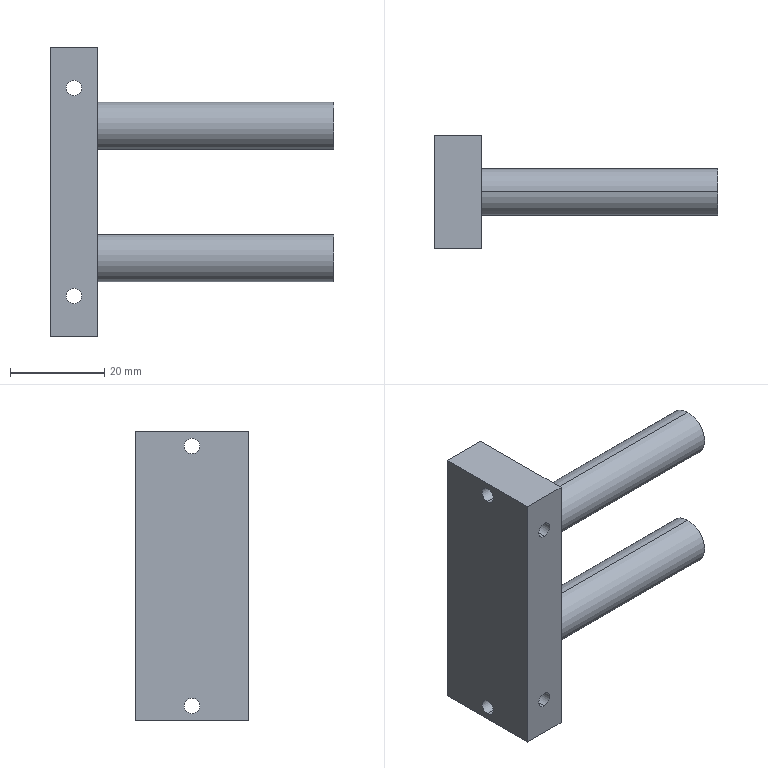Part | STEP file | PN_0013 cylinder TN-20X125 | 1 solid | 20 faces | box 60 x 24 x 61 mm | volume 21912 mm3 | cylinder 12 | plane 8 | commonest cylinder face diameters 3.3 x8 10 x4
STEP:
#1=CARTESIAN_POINT('',(0.,0.,0.));
#2=DIRECTION('',(0.,0.,1.));
#3=DIRECTION('',(1.,0.,0.));
#4=AXIS2_PLACEMENT_3D('',#1,#2,#3);
#5=CARTESIAN_POINT('',(0.,-12.,23.65));
#6=VERTEX_POINT('',#5);
#7=CARTESIAN_POINT('',(0.,12.,23.65));
#8=VERTEX_POINT('',#7);
#9=CARTESIAN_POINT('',(0.,12.,23.65));
#10=DIRECTION('',(0.,1.,0.));
#11=VECTOR('',#10,1.);
#12=LINE('',#9,#11);
#13=CARTESIAN_POINT('',(0.,12.,22.));
#14=DIRECTION('',(0.,1.,0.));
#15=DIRECTION('',(0.,0.,1.));
#16=AXIS2_PLACEMENT_3D('',#13,#14,#15);
#17=CYLINDRICAL_SURFACE('',#16,1.65);
#18=CARTESIAN_POINT('',(6.283,0.));
#19=DIRECTION('',(0.,1.));
#20=VECTOR('',#19,1.);
#21=LINE('',#18,#20);
#22=(GEOMETRIC_REPRESENTATION_CONTEXT(2)PARAMETRIC_REPRESENTATION_CONTEXT()REPRESENTATION_CONTEXT('',''));
#23=DEFINITIONAL_REPRESENTATION('',(#21),#22);
#24=PCURVE('',#17,#23);
#25=CARTESIAN_POINT('',(0.,12.,22.));
#26=DIRECTION('',(0.,1.,0.));
#27=DIRECTION('',(0.,0.,1.));
#28=AXIS2_PLACEMENT_3D('',#25,#26,#27);
#29=CYLINDRICAL_SURFACE('',#28,1.65);
#30=CARTESIAN_POINT('',(0.,0.));
#31=DIRECTION('',(0.,1.));
#32=VECTOR('',#31,1.);
#33=LINE('',#30,#32);
#34=(GEOMETRIC_REPRESENTATION_CONTEXT(2)PARAMETRIC_REPRESENTATION_CONTEXT()REPRESENTATION_CONTEXT('',''));
#35=DEFINITIONAL_REPRESENTATION('',(#33),#34);
#36=PCURVE('',#29,#35);
#37=SURFACE_CURVE('',#12,(#24,#36),.PCURVE_S1.);
#38=EDGE_CURVE('',#6,#8,#37,.T.);
#39=ORIENTED_EDGE('',*,*,#38,.T.);
#40=CARTESIAN_POINT('',(0.,12.,20.35));
#41=VERTEX_POINT('',#40);
#42=CARTESIAN_POINT('',(0.,12.,22.));
#43=DIRECTION('',(0.,1.,0.));
#44=DIRECTION('',(0.,0.,1.));
#45=AXIS2_PLACEMENT_3D('',#42,#43,#44);
#46=CIRCLE('',#45,1.65);
#47=CARTESIAN_POINT('',(0.,0.));
#48=DIRECTION('',(1.,0.));
#49=VECTOR('',#48,1.);
#50=LINE('',#47,#49);
#51=(GEOMETRIC_REPRESENTATION_CONTEXT(2)PARAMETRIC_REPRESENTATION_CONTEXT()REPRESENTATION_CONTEXT('',''));
#52=DEFINITIONAL_REPRESENTATION('',(#50),#51);
#53=PCURVE('',#17,#52);
#54=CARTESIAN_POINT('',(5.,12.,-30.5));
#55=DIRECTION('',(0.,-1.,0.));
#56=DIRECTION('',(0.,0.,-1.));
#57=AXIS2_PLACEMENT_3D('',#54,#55,#56);
#58=PLANE('',#57);
#59=CARTESIAN_POINT('',(-54.15,-5.));
#60=CARTESIAN_POINT('',(-54.15,-2.142));
#61=CARTESIAN_POINT('',(-51.675,-3.571));
#62=CARTESIAN_POINT('',(-49.2,-5.));
#63=CARTESIAN_POINT('',(-51.675,-6.429));
#64=CARTESIAN_POINT('',(-54.15,-7.858));
#65=CARTESIAN_POINT('',(-54.15,-5.));
#66=(BOUNDED_CURVE()B_SPLINE_CURVE(2,(#59,#60,#61,#62,#63,#64,#65),.UNSPECIFIED.,.T.,.F.)B_SPLINE_CURVE_WITH_KNOTS((1,2,2,2,2,1),(-2.094,0.,2.094,4.189,6.283,8.378),.UNSPECIFIED.)CURVE()GEOMETRIC_REPRESENTATION_ITEM()RATIONAL_B_SPLINE_CURVE((1.,0.5,1.,0.5,1.,0.5,1.))REPRESENTATION_ITEM(''));
#67=(GEOMETRIC_REPRESENTATION_CONTEXT(2)PARAMETRIC_REPRESENTATION_CONTEXT()REPRESENTATION_CONTEXT('',''));
#68=DEFINITIONAL_REPRESENTATION('',(#66),#67);
#69=PCURVE('',#58,#68);
#70=SURFACE_CURVE('',#46,(#53,#69),.PCURVE_S1.);
#71=EDGE_CURVE('',#41,#8,#70,.T.);
#72=ORIENTED_EDGE('',*,*,#71,.F.);
#73=CARTESIAN_POINT('',(0.,-12.,20.35));
#74=VERTEX_POINT('',#73);
#75=CARTESIAN_POINT('',(0.,12.,20.35));
#76=DIRECTION('',(0.,1.,0.));
#77=VECTOR('',#76,1.);
#78=LINE('',#75,#77);
#79=CARTESIAN_POINT('',(3.142,0.));
#80=DIRECTION('',(0.,1.));
#81=VECTOR('',#80,1.);
#82=LINE('',#79,#81);
#83=(GEOMETRIC_REPRESENTATION_CONTEXT(2)PARAMETRIC_REPRESENTATION_CONTEXT()REPRESENTATION_CONTEXT('',''));
#84=DEFINITIONAL_REPRESENTATION('',(#82),#83);
#85=PCURVE('',#17,#84);
#86=CARTESIAN_POINT('',(3.142,0.));
#87=DIRECTION('',(0.,1.));
#88=VECTOR('',#87,1.);
#89=LINE('',#86,#88);
#90=(GEOMETRIC_REPRESENTATION_CONTEXT(2)PARAMETRIC_REPRESENTATION_CONTEXT()REPRESENTATION_CONTEXT('',''));
#91=DEFINITIONAL_REPRESENTATION('',(#89),#90);
#92=PCURVE('',#29,#91);
#93=SURFACE_CURVE('',#78,(#85,#92),.PCURVE_S1.);
#94=EDGE_CURVE('',#74,#41,#93,.T.);
#95=ORIENTED_EDGE('',*,*,#94,.F.);
#96=CARTESIAN_POINT('',(0.,-12.,22.));
#97=DIRECTION('',(0.,1.,0.));
#98=DIRECTION('',(0.,0.,1.));
#99=AXIS2_PLACEMENT_3D('',#96,#97,#98);
#100=CIRCLE('',#99,1.65);
#101=CARTESIAN_POINT('',(0.,-24.));
#102=DIRECTION('',(1.,0.));
#103=VECTOR('',#102,1.);
#104=LINE('',#101,#103);
#105=(GEOMETRIC_REPRESENTATION_CONTEXT(2)PARAMETRIC_REPRESENTATION_CONTEXT()REPRESENTATION_CONTEXT('',''));
#106=DEFINITIONAL_REPRESENTATION('',(#104),#105);
#107=PCURVE('',#17,#106);
#108=CARTESIAN_POINT('',(5.,-12.,-30.5));
#109=DIRECTION('',(0.,1.,0.));
#110=DIRECTION('',(0.,0.,1.));
#111=AXIS2_PLACEMENT_3D('',#108,#109,#110);
#112=PLANE('',#111);
#113=CARTESIAN_POINT('',(52.5,-5.));
#114=DIRECTION('',(1.,0.));
#115=AXIS2_PLACEMENT_2D('',#113,#114);
#116=CIRCLE('',#115,1.65);
#117=(GEOMETRIC_REPRESENTATION_CONTEXT(2)PARAMETRIC_REPRESENTATION_CONTEXT()REPRESENTATION_CONTEXT('',''));
#118=DEFINITIONAL_REPRESENTATION('',(#116),#117);
#119=PCURVE('',#112,#118);
#120=SURFACE_CURVE('',#100,(#107,#119),.PCURVE_S1.);
#121=EDGE_CURVE('',#74,#6,#120,.T.);
#122=ORIENTED_EDGE('',*,*,#121,.T.);
#123=EDGE_LOOP('',(#39,#72,#95,#122));
#124=FACE_BOUND('',#123,.F.);
#125=ADVANCED_FACE('',(#124),#17,.F.);
#126=CARTESIAN_POINT('',(0.,-12.,-20.35));
#127=VERTEX_POINT('',#126);
#128=CARTESIAN_POINT('',(0.,12.,-20.35));
#129=VERTEX_POINT('',#128);
#130=CARTESIAN_POINT('',(0.,12.,-20.35));
#131=DIRECTION('',(0.,1.,0.));
#132=VECTOR('',#131,1.);
#133=LINE('',#130,#132);
#134=CARTESIAN_POINT('',(0.,12.,-22.));
#135=DIRECTION('',(0.,1.,0.));
#136=DIRECTION('',(0.,0.,1.));
#137=AXIS2_PLACEMENT_3D('',#134,#135,#136);
#138=CYLINDRICAL_SURFACE('',#137,1.65);
#139=CARTESIAN_POINT('',(6.283,0.));
#140=DIRECTION('',(0.,1.));
#141=VECTOR('',#140,1.);
#142=LINE('',#139,#141);
#143=(GEOMETRIC_REPRESENTATION_CONTEXT(2)PARAMETRIC_REPRESENTATION_CONTEXT()REPRESENTATION_CONTEXT('',''));
#144=DEFINITIONAL_REPRESENTATION('',(#142),#143);
#145=PCURVE('',#138,#144);
#146=CARTESIAN_POINT('',(0.,12.,-22.));
#147=DIRECTION('',(0.,1.,0.));
#148=DIRECTION('',(0.,0.,1.));
#149=AXIS2_PLACEMENT_3D('',#146,#147,#148);
#150=CYLINDRICAL_SURFACE('',#149,1.65);
#151=CARTESIAN_POINT('',(0.,0.));
#152=DIRECTION('',(0.,1.));
#153=VECTOR('',#152,1.);
#154=LINE('',#151,#153);
#155=(GEOMETRIC_REPRESENTATION_CONTEXT(2)PARAMETRIC_REPRESENTATION_CONTEXT()REPRESENTATION_CONTEXT('',''));
#156=DEFINITIONAL_REPRESENTATION('',(#154),#155);
#157=PCURVE('',#150,#156);
#158=SURFACE_CURVE('',#133,(#145,#157),.PCURVE_S1.);
#159=EDGE_CURVE('',#127,#129,#158,.T.);
#160=ORIENTED_EDGE('',*,*,#159,.T.);
#161=CARTESIAN_POINT('',(0.,12.,-23.65));
#162=VERTEX_POINT('',#161);
#163=CARTESIAN_POINT('',(0.,12.,-22.));
#164=DIRECTION('',(0.,1.,0.));
#165=DIRECTION('',(0.,0.,1.));
#166=AXIS2_PLACEMENT_3D('',#163,#164,#165);
#167=CIRCLE('',#166,1.65);
#168=CARTESIAN_POINT('',(0.,0.));
#169=DIRECTION('',(1.,0.));
#170=VECTOR('',#169,1.);
#171=LINE('',#168,#170);
#172=(GEOMETRIC_REPRESENTATION_CONTEXT(2)PARAMETRIC_REPRESENTATION_CONTEXT()REPRESENTATION_CONTEXT('',''));
#173=DEFINITIONAL_REPRESENTATION('',(#171),#172);
#174=PCURVE('',#138,#173);
#175=CARTESIAN_POINT('',(-10.15,-5.));
#176=CARTESIAN_POINT('',(-10.15,-2.142));
#177=CARTESIAN_POINT('',(-7.675,-3.571));
#178=CARTESIAN_POINT('',(-5.2,-5.));
#179=CARTESIAN_POINT('',(-7.675,-6.429));
#180=CARTESIAN_POINT('',(-10.15,-7.858));
#181=CARTESIAN_POINT('',(-10.15,-5.));
#182=(BOUNDED_CURVE()B_SPLINE_CURVE(2,(#175,#176,#177,#178,#179,#180,#181),.UNSPECIFIED.,.T.,.F.)B_SPLINE_CURVE_WITH_KNOTS((1,2,2,2,2,1),(-2.094,0.,2.094,4.189,6.283,8.378),.UNSPECIFIED.)CURVE()GEOMETRIC_REPRESENTATION_ITEM()RATIONAL_B_SPLINE_CURVE((1.,0.5,1.,0.5,1.,0.5,1.))REPRESENTATION_ITEM(''));
#183=(GEOMETRIC_REPRESENTATION_CONTEXT(2)PARAMETRIC_REPRESENTATION_CONTEXT()REPRESENTATION_CONTEXT('',''));
#184=DEFINITIONAL_REPRESENTATION('',(#182),#183);
#185=PCURVE('',#58,#184);
#186=SURFACE_CURVE('',#167,(#174,#185),.PCURVE_S1.);
#187=EDGE_CURVE('',#162,#129,#186,.T.);
#188=ORIENTED_EDGE('',*,*,#187,.F.);
#189=CARTESIAN_POINT('',(0.,-12.,-23.65));
#190=VERTEX_POINT('',#189);
#191=CARTESIAN_POINT('',(0.,12.,-23.65));
#192=DIRECTION('',(0.,1.,0.));
#193=VECTOR('',#192,1.);
#194=LINE('',#191,#193);
#195=CARTESIAN_POINT('',(3.142,0.));
#196=DIRECTION('',(0.,1.));
#197=VECTOR('',#196,1.);
#198=LINE('',#195,#197);
#199=(GEOMETRIC_REPRESENTATION_CONTEXT(2)PARAMETRIC_REPRESENTATION_CONTEXT()REPRESENTATION_CONTEXT('',''));
#200=DEFINITIONAL_REPRESENTATION('',(#198),#199);
#201=PCURVE('',#138,#200);
#202=CARTESIAN_POINT('',(3.142,0.));
#203=DIRECTION('',(0.,1.));
#204=VECTOR('',#203,1.);
#205=LINE('',#202,#204);
#206=(GEOMETRIC_REPRESENTATION_CONTEXT(2)PARAMETRIC_REPRESENTATION_CONTEXT()REPRESENTATION_CONTEXT('',''));
#207=DEFINITIONAL_REPRESENTATION('',(#205),#206);
#208=PCURVE('',#150,#207);
#209=SURFACE_CURVE('',#194,(#201,#208),.PCURVE_S1.);
#210=EDGE_CURVE('',#190,#162,#209,.T.);
#211=ORIENTED_EDGE('',*,*,#210,.F.);
#212=CARTESIAN_POINT('',(0.,-12.,-22.));
#213=DIRECTION('',(0.,1.,0.));
#214=DIRECTION('',(0.,0.,1.));
#215=AXIS2_PLACEMENT_3D('',#212,#213,#214);
#216=CIRCLE('',#215,1.65);
#217=CARTESIAN_POINT('',(0.,-24.));
#218=DIRECTION('',(1.,0.));
#219=VECTOR('',#218,1.);
#220=LINE('',#217,#219);
#221=(GEOMETRIC_REPRESENTATION_CONTEXT(2)PARAMETRIC_REPRESENTATION_CONTEXT()REPRESENTATION_CONTEXT('',''));
#222=DEFINITIONAL_REPRESENTATION('',(#220),#221);
#223=PCURVE('',#138,#222);
#224=CARTESIAN_POINT('',(8.5,-5.));
#225=DIRECTION('',(1.,0.));
#226=AXIS2_PLACEMENT_2D('',#224,#225);
#227=CIRCLE('',#226,1.65);
#228=(GEOMETRIC_REPRESENTATION_CONTEXT(2)PARAMETRIC_REPRESENTATION_CONTEXT()REPRESENTATION_CONTEXT('',''));
#229=DEFINITIONAL_REPRESENTATION('',(#227),#228);
#230=PCURVE('',#112,#229);
#231=SURFACE_CURVE('',#216,(#223,#230),.PCURVE_S1.);
#232=EDGE_CURVE('',#190,#127,#231,.T.);
#233=ORIENTED_EDGE('',*,*,#232,.T.);
#234=EDGE_LOOP('',(#160,#188,#211,#233));
#235=FACE_BOUND('',#234,.F.);
#236=ADVANCED_FACE('',(#235),#138,.F.);
#237=CARTESIAN_POINT('',(5.,0.,-25.85));
#238=VERTEX_POINT('',#237);
#239=CARTESIAN_POINT('',(-5.,0.,-25.85));
#240=VERTEX_POINT('',#239);
#241=CARTESIAN_POINT('',(-5.,0.,-25.85));
#242=DIRECTION('',(-1.,0.,0.));
#243=VECTOR('',#242,1.);
#244=LINE('',#241,#243);
#245=CARTESIAN_POINT('',(-5.,0.,-27.5));
#246=DIRECTION('',(-1.,0.,0.));
#247=DIRECTION('',(0.,0.,1.));
#248=AXIS2_PLACEMENT_3D('',#245,#246,#247);
#249=CYLINDRICAL_SURFACE('',#248,1.65);
#250=CARTESIAN_POINT('',(6.283,0.));
#251=DIRECTION('',(0.,1.));
#252=VECTOR('',#251,1.);
#253=LINE('',#250,#252);
#254=(GEOMETRIC_REPRESENTATION_CONTEXT(2)PARAMETRIC_REPRESENTATION_CONTEXT()REPRESENTATION_CONTEXT('',''));
#255=DEFINITIONAL_REPRESENTATION('',(#253),#254);
#256=PCURVE('',#249,#255);
#257=CARTESIAN_POINT('',(-5.,0.,-27.5));
#258=DIRECTION('',(-1.,0.,0.));
#259=DIRECTION('',(0.,0.,1.));
#260=AXIS2_PLACEMENT_3D('',#257,#258,#259);
#261=CYLINDRICAL_SURFACE('',#260,1.65);
#262=CARTESIAN_POINT('',(0.,0.));
#263=DIRECTION('',(0.,1.));
#264=VECTOR('',#263,1.);
#265=LINE('',#262,#264);
#266=(GEOMETRIC_REPRESENTATION_CONTEXT(2)PARAMETRIC_REPRESENTATION_CONTEXT()REPRESENTATION_CONTEXT('',''));
#267=DEFINITIONAL_REPRESENTATION('',(#265),#266);
#268=PCURVE('',#261,#267);
#269=SURFACE_CURVE('',#244,(#256,#268),.PCURVE_S1.);
#270=EDGE_CURVE('',#238,#240,#269,.T.);
#271=ORIENTED_EDGE('',*,*,#270,.T.);
#272=CARTESIAN_POINT('',(-5.,0.,-29.15));
#273=VERTEX_POINT('',#272);
#274=CARTESIAN_POINT('',(-5.,0.,-27.5));
#275=DIRECTION('',(-1.,0.,0.));
#276=DIRECTION('',(0.,0.,1.));
#277=AXIS2_PLACEMENT_3D('',#274,#275,#276);
#278=CIRCLE('',#277,1.65);
#279=CARTESIAN_POINT('',(0.,0.));
#280=DIRECTION('',(1.,0.));
#281=VECTOR('',#280,1.);
#282=LINE('',#279,#281);
#283=(GEOMETRIC_REPRESENTATION_CONTEXT(2)PARAMETRIC_REPRESENTATION_CONTEXT()REPRESENTATION_CONTEXT('',''));
#284=DEFINITIONAL_REPRESENTATION('',(#282),#283);
#285=PCURVE('',#249,#284);
#286=CARTESIAN_POINT('',(-5.,0.,0.));
#287=DIRECTION('',(1.,0.,0.));
#288=DIRECTION('',(0.,0.,-1.));
#289=AXIS2_PLACEMENT_3D('',#286,#287,#288);
#290=PLANE('',#289);
#291=CARTESIAN_POINT('',(25.85,0.));
#292=CARTESIAN_POINT('',(25.85,2.858));
#293=CARTESIAN_POINT('',(28.325,1.429));
#294=CARTESIAN_POINT('',(30.8,0.));
#295=CARTESIAN_POINT('',(28.325,-1.429));
#296=CARTESIAN_POINT('',(25.85,-2.858));
#297=CARTESIAN_POINT('',(25.85,0.));
#298=(BOUNDED_CURVE()B_SPLINE_CURVE(2,(#291,#292,#293,#294,#295,#296,#297),.UNSPECIFIED.,.T.,.F.)B_SPLINE_CURVE_WITH_KNOTS((1,2,2,2,2,1),(-2.094,0.,2.094,4.189,6.283,8.378),.UNSPECIFIED.)CURVE()GEOMETRIC_REPRESENTATION_ITEM()RATIONAL_B_SPLINE_CURVE((1.,0.5,1.,0.5,1.,0.5,1.))REPRESENTATION_ITEM(''));
#299=(GEOMETRIC_REPRESENTATION_CONTEXT(2)PARAMETRIC_REPRESENTATION_CONTEXT()REPRESENTATION_CONTEXT('',''));
#300=DEFINITIONAL_REPRESENTATION('',(#298),#299);
#301=PCURVE('',#290,#300);
#302=SURFACE_CURVE('',#278,(#285,#301),.PCURVE_S1.);
#303=EDGE_CURVE('',#273,#240,#302,.T.);
#304=ORIENTED_EDGE('',*,*,#303,.F.);
#305=CARTESIAN_POINT('',(5.,0.,-29.15));
#306=VERTEX_POINT('',#305);
#307=CARTESIAN_POINT('',(-5.,0.,-29.15));
#308=DIRECTION('',(-1.,0.,0.));
#309=VECTOR('',#308,1.);
#310=LINE('',#307,#309);
#311=CARTESIAN_POINT('',(3.142,0.));
#312=DIRECTION('',(0.,1.));
#313=VECTOR('',#312,1.);
#314=LINE('',#311,#313);
#315=(GEOMETRIC_REPRESENTATION_CONTEXT(2)PARAMETRIC_REPRESENTATION_CONTEXT()REPRESENTATION_CONTEXT('',''));
#316=DEFINITIONAL_REPRESENTATION('',(#314),#315);
#317=PCURVE('',#249,#316);
#318=CARTESIAN_POINT('',(3.142,0.));
#319=DIRECTION('',(0.,1.));
#320=VECTOR('',#319,1.);
#321=LINE('',#318,#320);
#322=(GEOMETRIC_REPRESENTATION_CONTEXT(2)PARAMETRIC_REPRESENTATION_CONTEXT()REPRESENTATION_CONTEXT('',''));
#323=DEFINITIONAL_REPRESENTATION('',(#321),#322);
#324=PCURVE('',#261,#323);
#325=SURFACE_CURVE('',#310,(#317,#324),.PCURVE_S1.);
#326=EDGE_CURVE('',#306,#273,#325,.T.);
#327=ORIENTED_EDGE('',*,*,#326,.F.);
#328=CARTESIAN_POINT('',(5.,0.,-27.5));
#329=DIRECTION('',(1.,0.,0.));
#330=DIRECTION('',(0.,0.,-1.));
#331=AXIS2_PLACEMENT_3D('',#328,#329,#330);
#332=CIRCLE('',#331,1.65);
#333=CARTESIAN_POINT('',(9.425,-10.));
#334=DIRECTION('',(-1.,0.));
#335=VECTOR('',#334,1.);
#336=LINE('',#333,#335);
#337=(GEOMETRIC_REPRESENTATION_CONTEXT(2)PARAMETRIC_REPRESENTATION_CONTEXT()REPRESENTATION_CONTEXT('',''));
#338=DEFINITIONAL_REPRESENTATION('',(#336),#337);
#339=PCURVE('',#249,#338);
#340=CARTESIAN_POINT('',(5.,0.,0.));
#341=DIRECTION('',(1.,0.,0.));
#342=DIRECTION('',(0.,0.,-1.));
#343=AXIS2_PLACEMENT_3D('',#340,#341,#342);
#344=PLANE('',#343);
#345=CARTESIAN_POINT('',(27.5,0.));
#346=DIRECTION('',(1.,0.));
#347=AXIS2_PLACEMENT_2D('',#345,#346);
#348=CIRCLE('',#347,1.65);
#349=(GEOMETRIC_REPRESENTATION_CONTEXT(2)PARAMETRIC_REPRESENTATION_CONTEXT()REPRESENTATION_CONTEXT('',''));
#350=DEFINITIONAL_REPRESENTATION('',(#348),#349);
#351=PCURVE('',#344,#350);
#352=SURFACE_CURVE('',#332,(#339,#351),.PCURVE_S1.);
#353=EDGE_CURVE('',#238,#306,#352,.T.);
#354=ORIENTED_EDGE('',*,*,#353,.F.);
#355=EDGE_LOOP('',(#271,#304,#327,#354));
#356=FACE_BOUND('',#355,.F.);
#357=ADVANCED_FACE('',(#356),#249,.F.);
#358=CARTESIAN_POINT('',(5.,0.,29.15));
#359=VERTEX_POINT('',#358);
#360=CARTESIAN_POINT('',(-5.,0.,29.15));
#361=VERTEX_POINT('',#360);
#362=CARTESIAN_POINT('',(-5.,0.,29.15));
#363=DIRECTION('',(-1.,0.,0.));
#364=VECTOR('',#363,1.);
#365=LINE('',#362,#364);
#366=CARTESIAN_POINT('',(-5.,0.,27.5));
#367=DIRECTION('',(-1.,0.,0.));
#368=DIRECTION('',(0.,0.,1.));
#369=AXIS2_PLACEMENT_3D('',#366,#367,#368);
#370=CYLINDRICAL_SURFACE('',#369,1.65);
#371=CARTESIAN_POINT('',(6.283,0.));
#372=DIRECTION('',(0.,1.));
#373=VECTOR('',#372,1.);
#374=LINE('',#371,#373);
#375=(GEOMETRIC_REPRESENTATION_CONTEXT(2)PARAMETRIC_REPRESENTATION_CONTEXT()REPRESENTATION_CONTEXT('',''));
#376=DEFINITIONAL_REPRESENTATION('',(#374),#375);
#377=PCURVE('',#370,#376);
#378=CARTESIAN_POINT('',(-5.,0.,27.5));
#379=DIRECTION('',(-1.,0.,0.));
#380=DIRECTION('',(0.,0.,1.));
#381=AXIS2_PLACEMENT_3D('',#378,#379,#380);
#382=CYLINDRICAL_SURFACE('',#381,1.65);
#383=CARTESIAN_POINT('',(0.,0.));
#384=DIRECTION('',(0.,1.));
#385=VECTOR('',#384,1.);
#386=LINE('',#383,#385);
#387=(GEOMETRIC_REPRESENTATION_CONTEXT(2)PARAMETRIC_REPRESENTATION_CONTEXT()REPRESENTATION_CONTEXT('',''));
#388=DEFINITIONAL_REPRESENTATION('',(#386),#387);
#389=PCURVE('',#382,#388);
#390=SURFACE_CURVE('',#365,(#377,#389),.PCURVE_S1.);
#391=EDGE_CURVE('',#359,#361,#390,.T.);
#392=ORIENTED_EDGE('',*,*,#391,.T.);
#393=CARTESIAN_POINT('',(-5.,0.,25.85));
#394=VERTEX_POINT('',#393);
#395=CARTESIAN_POINT('',(-5.,0.,27.5));
#396=DIRECTION('',(-1.,0.,0.));
#397=DIRECTION('',(0.,0.,1.));
#398=AXIS2_PLACEMENT_3D('',#395,#396,#397);
#399=CIRCLE('',#398,1.65);
#400=CARTESIAN_POINT('',(0.,0.));
#401=DIRECTION('',(1.,0.));
#402=VECTOR('',#401,1.);
#403=LINE('',#400,#402);
#404=(GEOMETRIC_REPRESENTATION_CONTEXT(2)PARAMETRIC_REPRESENTATION_CONTEXT()REPRESENTATION_CONTEXT('',''));
#405=DEFINITIONAL_REPRESENTATION('',(#403),#404);
#406=PCURVE('',#370,#405);
#407=CARTESIAN_POINT('',(-29.15,0.));
#408=CARTESIAN_POINT('',(-29.15,2.858));
#409=CARTESIAN_POINT('',(-26.675,1.429));
#410=CARTESIAN_POINT('',(-24.2,0.));
#411=CARTESIAN_POINT('',(-26.675,-1.429));
#412=CARTESIAN_POINT('',(-29.15,-2.858));
#413=CARTESIAN_POINT('',(-29.15,0.));
#414=(BOUNDED_CURVE()B_SPLINE_CURVE(2,(#407,#408,#409,#410,#411,#412,#413),.UNSPECIFIED.,.T.,.F.)B_SPLINE_CURVE_WITH_KNOTS((1,2,2,2,2,1),(-2.094,0.,2.094,4.189,6.283,8.378),.UNSPECIFIED.)CURVE()GEOMETRIC_REPRESENTATION_ITEM()RATIONAL_B_SPLINE_CURVE((1.,0.5,1.,0.5,1.,0.5,1.))REPRESENTATION_ITEM(''));
#415=(GEOMETRIC_REPRESENTATION_CONTEXT(2)PARAMETRIC_REPRESENTATION_CONTEXT()REPRESENTATION_CONTEXT('',''));
#416=DEFINITIONAL_REPRESENTATION('',(#414),#415);
#417=PCURVE('',#290,#416);
#418=SURFACE_CURVE('',#399,(#406,#417),.PCURVE_S1.);
#419=EDGE_CURVE('',#394,#361,#418,.T.);
#420=ORIENTED_EDGE('',*,*,#419,.F.);
#421=CARTESIAN_POINT('',(5.,0.,25.85));
#422=VERTEX_POINT('',#421);
#423=CARTESIAN_POINT('',(-5.,0.,25.85));
#424=DIRECTION('',(-1.,0.,0.));
#425=VECTOR('',#424,1.);
#426=LINE('',#423,#425);
#427=CARTESIAN_POINT('',(3.142,0.));
#428=DIRECTION('',(0.,1.));
#429=VECTOR('',#428,1.);
#430=LINE('',#427,#429);
#431=(GEOMETRIC_REPRESENTATION_CONTEXT(2)PARAMETRIC_REPRESENTATION_CONTEXT()REPRESENTATION_CONTEXT('',''));
#432=DEFINITIONAL_REPRESENTATION('',(#430),#431);
#433=PCURVE('',#370,#432);
#434=CARTESIAN_POINT('',(3.142,0.));
#435=DIRECTION('',(0.,1.));
#436=VECTOR('',#435,1.);
#437=LINE('',#434,#436);
#438=(GEOMETRIC_REPRESENTATION_CONTEXT(2)PARAMETRIC_REPRESENTATION_CONTEXT()REPRESENTATION_CONTEXT('',''));
#439=DEFINITIONAL_REPRESENTATION('',(#437),#438);
#440=PCURVE('',#382,#439);
#441=SURFACE_CURVE('',#426,(#433,#440),.PCURVE_S1.);
#442=EDGE_CURVE('',#422,#394,#441,.T.);
#443=ORIENTED_EDGE('',*,*,#442,.F.);
#444=CARTESIAN_POINT('',(5.,0.,27.5));
#445=DIRECTION('',(1.,0.,0.));
#446=DIRECTION('',(0.,0.,-1.));
#447=AXIS2_PLACEMENT_3D('',#444,#445,#446);
#448=CIRCLE('',#447,1.65);
#449=CARTESIAN_POINT('',(9.425,-10.));
#450=DIRECTION('',(-1.,0.));
#451=VECTOR('',#450,1.);
#452=LINE('',#449,#451);
#453=(GEOMETRIC_REPRESENTATION_CONTEXT(2)PARAMETRIC_REPRESENTATION_CONTEXT()REPRESENTATION_CONTEXT('',''));
#454=DEFINITIONAL_REPRESENTATION('',(#452),#453);
#455=PCURVE('',#370,#454);
#456=CARTESIAN_POINT('',(-27.5,0.));
#457=DIRECTION('',(1.,0.));
#458=AXIS2_PLACEMENT_2D('',#456,#457);
#459=CIRCLE('',#458,1.65);
#460=(GEOMETRIC_REPRESENTATION_CONTEXT(2)PARAMETRIC_REPRESENTATION_CONTEXT()REPRESENTATION_CONTEXT('',''));
#461=DEFINITIONAL_REPRESENTATION('',(#459),#460);
#462=PCURVE('',#344,#461);
#463=SURFACE_CURVE('',#448,(#455,#462),.PCURVE_S1.);
#464=EDGE_CURVE('',#359,#422,#463,.T.);
#465=ORIENTED_EDGE('',*,*,#464,.F.);
#466=EDGE_LOOP('',(#392,#420,#443,#465));
#467=FACE_BOUND('',#466,.F.);
#468=ADVANCED_FACE('',(#467),#370,.F.);
#469=CARTESIAN_POINT('',(55.,0.,-19.));
#470=VERTEX_POINT('',#469);
#471=CARTESIAN_POINT('',(55.,0.,-9.));
#472=VERTEX_POINT('',#471);
#473=CARTESIAN_POINT('',(55.,0.,-14.));
#474=DIRECTION('',(1.,0.,0.));
#475=DIRECTION('',(0.,0.,-1.));
#476=AXIS2_PLACEMENT_3D('',#473,#474,#475);
#477=CIRCLE('',#476,5.);
#478=CARTESIAN_POINT('',(55.,0.,-14.));
#479=DIRECTION('',(-1.,0.,0.));
#480=DIRECTION('',(0.,0.,1.));
#481=AXIS2_PLACEMENT_3D('',#478,#479,#480);
#482=CYLINDRICAL_SURFACE('',#481,5.);
#483=CARTESIAN_POINT('',(3.142,0.));
#484=DIRECTION('',(-1.,0.));
#485=VECTOR('',#484,1.);
#486=LINE('',#483,#485);
#487=(GEOMETRIC_REPRESENTATION_CONTEXT(2)PARAMETRIC_REPRESENTATION_CONTEXT()REPRESENTATION_CONTEXT('',''));
#488=DEFINITIONAL_REPRESENTATION('',(#486),#487);
#489=PCURVE('',#482,#488);
#490=CARTESIAN_POINT('',(55.,0.,-14.));
#491=DIRECTION('',(1.,0.,0.));
#492=DIRECTION('',(0.,0.,-1.));
#493=AXIS2_PLACEMENT_3D('',#490,#491,#492);
#494=PLANE('',#493);
#495=CARTESIAN_POINT('',(0.,0.));
#496=DIRECTION('',(1.,0.));
#497=AXIS2_PLACEMENT_2D('',#495,#496);
#498=CIRCLE('',#497,5.);
#499=(GEOMETRIC_REPRESENTATION_CONTEXT(2)PARAMETRIC_REPRESENTATION_CONTEXT()REPRESENTATION_CONTEXT('',''));
#500=DEFINITIONAL_REPRESENTATION('',(#498),#499);
#501=PCURVE('',#494,#500);
#502=SURFACE_CURVE('',#477,(#489,#501),.PCURVE_S1.);
#503=EDGE_CURVE('',#470,#472,#502,.T.);
#504=ORIENTED_EDGE('',*,*,#503,.F.);
#505=CARTESIAN_POINT('',(5.,0.,-19.));
#506=VERTEX_POINT('',#505);
#507=CARTESIAN_POINT('',(55.,0.,-19.));
#508=DIRECTION('',(-1.,0.,0.));
#509=VECTOR('',#508,1.);
#510=LINE('',#507,#509);
#511=CARTESIAN_POINT('',(3.142,0.));
#512=DIRECTION('',(0.,1.));
#513=VECTOR('',#512,1.);
#514=LINE('',#511,#513);
#515=(GEOMETRIC_REPRESENTATION_CONTEXT(2)PARAMETRIC_REPRESENTATION_CONTEXT()REPRESENTATION_CONTEXT('',''));
#516=DEFINITIONAL_REPRESENTATION('',(#514),#515);
#517=PCURVE('',#482,#516);
#518=CARTESIAN_POINT('',(55.,0.,-14.));
#519=DIRECTION('',(-1.,0.,0.));
#520=DIRECTION('',(0.,0.,1.));
#521=AXIS2_PLACEMENT_3D('',#518,#519,#520);
#522=CYLINDRICAL_SURFACE('',#521,5.);
#523=CARTESIAN_POINT('',(3.142,0.));
#524=DIRECTION('',(0.,1.));
#525=VECTOR('',#524,1.);
#526=LINE('',#523,#525);
#527=(GEOMETRIC_REPRESENTATION_CONTEXT(2)PARAMETRIC_REPRESENTATION_CONTEXT()REPRESENTATION_CONTEXT('',''));
#528=DEFINITIONAL_REPRESENTATION('',(#526),#527);
#529=PCURVE('',#522,#528);
#530=SURFACE_CURVE('',#510,(#517,#529),.PCURVE_S1.);
#531=EDGE_CURVE('',#470,#506,#530,.T.);
#532=ORIENTED_EDGE('',*,*,#531,.T.);
#533=CARTESIAN_POINT('',(5.,0.,-9.));
#534=VERTEX_POINT('',#533);
#535=CARTESIAN_POINT('',(5.,0.,-14.));
#536=DIRECTION('',(1.,0.,0.));
#537=DIRECTION('',(0.,0.,-1.));
#538=AXIS2_PLACEMENT_3D('',#535,#536,#537);
#539=CIRCLE('',#538,5.);
#540=CARTESIAN_POINT('',(3.142,50.));
#541=DIRECTION('',(-1.,0.));
#542=VECTOR('',#541,1.);
#543=LINE('',#540,#542);
#544=(GEOMETRIC_REPRESENTATION_CONTEXT(2)PARAMETRIC_REPRESENTATION_CONTEXT()REPRESENTATION_CONTEXT('',''));
#545=DEFINITIONAL_REPRESENTATION('',(#543),#544);
#546=PCURVE('',#482,#545);
#547=CARTESIAN_POINT('',(14.,0.));
#548=DIRECTION('',(1.,0.));
#549=AXIS2_PLACEMENT_2D('',#547,#548);
#550=CIRCLE('',#549,5.);
#551=(GEOMETRIC_REPRESENTATION_CONTEXT(2)PARAMETRIC_REPRESENTATION_CONTEXT()REPRESENTATION_CONTEXT('',''));
#552=DEFINITIONAL_REPRESENTATION('',(#550),#551);
#553=PCURVE('',#344,#552);
#554=SURFACE_CURVE('',#539,(#546,#553),.PCURVE_S1.);
#555=EDGE_CURVE('',#506,#534,#554,.T.);
#556=ORIENTED_EDGE('',*,*,#555,.T.);
#557=CARTESIAN_POINT('',(55.,0.,-9.));
#558=DIRECTION('',(-1.,0.,0.));
#559=VECTOR('',#558,1.);
#560=LINE('',#557,#559);
#561=CARTESIAN_POINT('',(0.,0.));
#562=DIRECTION('',(0.,1.));
#563=VECTOR('',#562,1.);
#564=LINE('',#561,#563);
#565=(GEOMETRIC_REPRESENTATION_CONTEXT(2)PARAMETRIC_REPRESENTATION_CONTEXT()REPRESENTATION_CONTEXT('',''));
#566=DEFINITIONAL_REPRESENTATION('',(#564),#565);
#567=PCURVE('',#482,#566);
#568=CARTESIAN_POINT('',(6.283,0.));
#569=DIRECTION('',(0.,1.));
#570=VECTOR('',#569,1.);
#571=LINE('',#568,#570);
#572=(GEOMETRIC_REPRESENTATION_CONTEXT(2)PARAMETRIC_REPRESENTATION_CONTEXT()REPRESENTATION_CONTEXT('',''));
#573=DEFINITIONAL_REPRESENTATION('',(#571),#572);
#574=PCURVE('',#522,#573);
#575=SURFACE_CURVE('',#560,(#567,#574),.PCURVE_S1.);
#576=EDGE_CURVE('',#472,#534,#575,.T.);
#577=ORIENTED_EDGE('',*,*,#576,.F.);
#578=EDGE_LOOP('',(#504,#532,#556,#577));
#579=FACE_BOUND('',#578,.T.);
#580=ADVANCED_FACE('',(#579),#482,.T.);
#581=CARTESIAN_POINT('',(55.,0.,9.));
#582=VERTEX_POINT('',#581);
#583=CARTESIAN_POINT('',(55.,0.,19.));
#584=VERTEX_POINT('',#583);
#585=CARTESIAN_POINT('',(55.,0.,14.));
#586=DIRECTION('',(1.,0.,0.));
#587=DIRECTION('',(0.,0.,-1.));
#588=AXIS2_PLACEMENT_3D('',#585,#586,#587);
#589=CIRCLE('',#588,5.);
#590=CARTESIAN_POINT('',(55.,0.,14.));
#591=DIRECTION('',(-1.,0.,0.));
#592=DIRECTION('',(0.,0.,1.));
#593=AXIS2_PLACEMENT_3D('',#590,#591,#592);
#594=CYLINDRICAL_SURFACE('',#593,5.);
#595=CARTESIAN_POINT('',(3.142,0.));
#596=DIRECTION('',(-1.,0.));
#597=VECTOR('',#596,1.);
#598=LINE('',#595,#597);
#599=(GEOMETRIC_REPRESENTATION_CONTEXT(2)PARAMETRIC_REPRESENTATION_CONTEXT()REPRESENTATION_CONTEXT('',''));
#600=DEFINITIONAL_REPRESENTATION('',(#598),#599);
#601=PCURVE('',#594,#600);
#602=CARTESIAN_POINT('',(55.,0.,14.));
#603=DIRECTION('',(1.,0.,0.));
#604=DIRECTION('',(0.,0.,-1.));
#605=AXIS2_PLACEMENT_3D('',#602,#603,#604);
#606=PLANE('',#605);
#607=CARTESIAN_POINT('',(0.,0.));
#608=DIRECTION('',(1.,0.));
#609=AXIS2_PLACEMENT_2D('',#607,#608);
#610=CIRCLE('',#609,5.);
#611=(GEOMETRIC_REPRESENTATION_CONTEXT(2)PARAMETRIC_REPRESENTATION_CONTEXT()REPRESENTATION_CONTEXT('',''));
#612=DEFINITIONAL_REPRESENTATION('',(#610),#611);
#613=PCURVE('',#606,#612);
#614=SURFACE_CURVE('',#589,(#601,#613),.PCURVE_S1.);
#615=EDGE_CURVE('',#582,#584,#614,.T.);
#616=ORIENTED_EDGE('',*,*,#615,.F.);
#617=CARTESIAN_POINT('',(5.,0.,9.));
#618=VERTEX_POINT('',#617);
#619=CARTESIAN_POINT('',(55.,0.,9.));
#620=DIRECTION('',(-1.,0.,0.));
#621=VECTOR('',#620,1.);
#622=LINE('',#619,#621);
#623=CARTESIAN_POINT('',(3.142,0.));
#624=DIRECTION('',(0.,1.));
#625=VECTOR('',#624,1.);
#626=LINE('',#623,#625);
#627=(GEOMETRIC_REPRESENTATION_CONTEXT(2)PARAMETRIC_REPRESENTATION_CONTEXT()REPRESENTATION_CONTEXT('',''));
#628=DEFINITIONAL_REPRESENTATION('',(#626),#627);
#629=PCURVE('',#594,#628);
#630=CARTESIAN_POINT('',(55.,0.,14.));
#631=DIRECTION('',(-1.,0.,0.));
#632=DIRECTION('',(0.,0.,1.));
#633=AXIS2_PLACEMENT_3D('',#630,#631,#632);
#634=CYLINDRICAL_SURFACE('',#633,5.);
#635=CARTESIAN_POINT('',(3.142,0.));
#636=DIRECTION('',(0.,1.));
#637=VECTOR('',#636,1.);
#638=LINE('',#635,#637);
#639=(GEOMETRIC_REPRESENTATION_CONTEXT(2)PARAMETRIC_REPRESENTATION_CONTEXT()REPRESENTATION_CONTEXT('',''));
#640=DEFINITIONAL_REPRESENTATION('',(#638),#639);
#641=PCURVE('',#634,#640);
#642=SURFACE_CURVE('',#622,(#629,#641),.PCURVE_S1.);
#643=EDGE_CURVE('',#582,#618,#642,.T.);
#644=ORIENTED_EDGE('',*,*,#643,.T.);
#645=CARTESIAN_POINT('',(5.,0.,19.));
#646=VERTEX_POINT('',#645);
#647=CARTESIAN_POINT('',(5.,0.,14.));
#648=DIRECTION('',(1.,0.,0.));
#649=DIRECTION('',(0.,0.,-1.));
#650=AXIS2_PLACEMENT_3D('',#647,#648,#649);
#651=CIRCLE('',#650,5.);
#652=CARTESIAN_POINT('',(3.142,50.));
#653=DIRECTION('',(-1.,0.));
#654=VECTOR('',#653,1.);
#655=LINE('',#652,#654);
#656=(GEOMETRIC_REPRESENTATION_CONTEXT(2)PARAMETRIC_REPRESENTATION_CONTEXT()REPRESENTATION_CONTEXT('',''));
#657=DEFINITIONAL_REPRESENTATION('',(#655),#656);
#658=PCURVE('',#594,#657);
#659=CARTESIAN_POINT('',(-14.,0.));
#660=DIRECTION('',(1.,0.));
#661=AXIS2_PLACEMENT_2D('',#659,#660);
#662=CIRCLE('',#661,5.);
#663=(GEOMETRIC_REPRESENTATION_CONTEXT(2)PARAMETRIC_REPRESENTATION_CONTEXT()REPRESENTATION_CONTEXT('',''));
#664=DEFINITIONAL_REPRESENTATION('',(#662),#663);
#665=PCURVE('',#344,#664);
#666=SURFACE_CURVE('',#651,(#658,#665),.PCURVE_S1.);
#667=EDGE_CURVE('',#618,#646,#666,.T.);
#668=ORIENTED_EDGE('',*,*,#667,.T.);
#669=CARTESIAN_POINT('',(55.,0.,19.));
#670=DIRECTION('',(-1.,0.,0.));
#671=VECTOR('',#670,1.);
#672=LINE('',#669,#671);
#673=CARTESIAN_POINT('',(0.,0.));
#674=DIRECTION('',(0.,1.));
#675=VECTOR('',#674,1.);
#676=LINE('',#673,#675);
#677=(GEOMETRIC_REPRESENTATION_CONTEXT(2)PARAMETRIC_REPRESENTATION_CONTEXT()REPRESENTATION_CONTEXT('',''));
#678=DEFINITIONAL_REPRESENTATION('',(#676),#677);
#679=PCURVE('',#594,#678);
#680=CARTESIAN_POINT('',(6.283,0.));
#681=DIRECTION('',(0.,1.));
#682=VECTOR('',#681,1.);
#683=LINE('',#680,#682);
#684=(GEOMETRIC_REPRESENTATION_CONTEXT(2)PARAMETRIC_REPRESENTATION_CONTEXT()REPRESENTATION_CONTEXT('',''));
#685=DEFINITIONAL_REPRESENTATION('',(#683),#684);
#686=PCURVE('',#634,#685);
#687=SURFACE_CURVE('',#672,(#679,#686),.PCURVE_S1.);
#688=EDGE_CURVE('',#584,#646,#687,.T.);
#689=ORIENTED_EDGE('',*,*,#688,.F.);
#690=EDGE_LOOP('',(#616,#644,#668,#689));
#691=FACE_BOUND('',#690,.T.);
#692=ADVANCED_FACE('',(#691),#594,.T.);
#693=ORIENTED_EDGE('',*,*,#353,.F.);
#694=CARTESIAN_POINT('',(5.,0.,-27.5));
#695=DIRECTION('',(1.,0.,0.));
#696=DIRECTION('',(0.,0.,-1.));
#697=AXIS2_PLACEMENT_3D('',#694,#695,#696);
#698=CIRCLE('',#697,1.65);
#699=CARTESIAN_POINT('',(27.5,0.));
#700=DIRECTION('',(1.,0.));
#701=AXIS2_PLACEMENT_2D('',#699,#700);
#702=CIRCLE('',#701,1.65);
#703=(GEOMETRIC_REPRESENTATION_CONTEXT(2)PARAMETRIC_REPRESENTATION_CONTEXT()REPRESENTATION_CONTEXT('',''));
#704=DEFINITIONAL_REPRESENTATION('',(#702),#703);
#705=PCURVE('',#344,#704);
#706=CARTESIAN_POINT('',(3.142,-10.));
#707=DIRECTION('',(-1.,0.));
#708=VECTOR('',#707,1.);
#709=LINE('',#706,#708);
#710=(GEOMETRIC_REPRESENTATION_CONTEXT(2)PARAMETRIC_REPRESENTATION_CONTEXT()REPRESENTATION_CONTEXT('',''));
#711=DEFINITIONAL_REPRESENTATION('',(#709),#710);
#712=PCURVE('',#261,#711);
#713=SURFACE_CURVE('',#698,(#705,#712),.PCURVE_S1.);
#714=EDGE_CURVE('',#306,#238,#713,.T.);
#715=ORIENTED_EDGE('',*,*,#714,.F.);
#716=EDGE_LOOP('',(#693,#715));
#717=FACE_BOUND('',#716,.T.);
#718=ORIENTED_EDGE('',*,*,#464,.F.);
#719=CARTESIAN_POINT('',(5.,0.,27.5));
#720=DIRECTION('',(1.,0.,0.));
#721=DIRECTION('',(0.,0.,-1.));
#722=AXIS2_PLACEMENT_3D('',#719,#720,#721);
#723=CIRCLE('',#722,1.65);
#724=CARTESIAN_POINT('',(-27.5,0.));
#725=DIRECTION('',(1.,0.));
#726=AXIS2_PLACEMENT_2D('',#724,#725);
#727=CIRCLE('',#726,1.65);
#728=(GEOMETRIC_REPRESENTATION_CONTEXT(2)PARAMETRIC_REPRESENTATION_CONTEXT()REPRESENTATION_CONTEXT('',''));
#729=DEFINITIONAL_REPRESENTATION('',(#727),#728);
#730=PCURVE('',#344,#729);
#731=CARTESIAN_POINT('',(3.142,-10.));
#732=DIRECTION('',(-1.,0.));
#733=VECTOR('',#732,1.);
#734=LINE('',#731,#733);
#735=(GEOMETRIC_REPRESENTATION_CONTEXT(2)PARAMETRIC_REPRESENTATION_CONTEXT()REPRESENTATION_CONTEXT('',''));
#736=DEFINITIONAL_REPRESENTATION('',(#734),#735);
#737=PCURVE('',#382,#736);
#738=SURFACE_CURVE('',#723,(#730,#737),.PCURVE_S1.);
#739=EDGE_CURVE('',#422,#359,#738,.T.);
#740=ORIENTED_EDGE('',*,*,#739,.F.);
#741=EDGE_LOOP('',(#718,#740));
#742=FACE_BOUND('',#741,.T.);
#743=CARTESIAN_POINT('',(5.,0.,14.));
#744=DIRECTION('',(1.,0.,0.));
#745=DIRECTION('',(0.,0.,-1.));
#746=AXIS2_PLACEMENT_3D('',#743,#744,#745);
#747=CIRCLE('',#746,5.);
#748=CARTESIAN_POINT('',(-14.,0.));
#749=DIRECTION('',(1.,0.));
#750=AXIS2_PLACEMENT_2D('',#748,#749);
#751=CIRCLE('',#750,5.);
#752=(GEOMETRIC_REPRESENTATION_CONTEXT(2)PARAMETRIC_REPRESENTATION_CONTEXT()REPRESENTATION_CONTEXT('',''));
#753=DEFINITIONAL_REPRESENTATION('',(#751),#752);
#754=PCURVE('',#344,#753);
#755=CARTESIAN_POINT('',(9.425,50.));
#756=DIRECTION('',(-1.,0.));
#757=VECTOR('',#756,1.);
#758=LINE('',#755,#757);
#759=(GEOMETRIC_REPRESENTATION_CONTEXT(2)PARAMETRIC_REPRESENTATION_CONTEXT()REPRESENTATION_CONTEXT('',''));
#760=DEFINITIONAL_REPRESENTATION('',(#758),#759);
#761=PCURVE('',#634,#760);
#762=SURFACE_CURVE('',#747,(#754,#761),.PCURVE_S1.);
#763=EDGE_CURVE('',#646,#618,#762,.T.);
#764=ORIENTED_EDGE('',*,*,#763,.F.);
#765=ORIENTED_EDGE('',*,*,#667,.F.);
#766=EDGE_LOOP('',(#764,#765));
#767=FACE_BOUND('',#766,.T.);
#768=CARTESIAN_POINT('',(5.,12.,30.5));
#769=VERTEX_POINT('',#768);
#770=CARTESIAN_POINT('',(5.,-12.,30.5));
#771=VERTEX_POINT('',#770);
#772=CARTESIAN_POINT('',(5.,-12.,30.5));
#773=DIRECTION('',(0.,-1.,0.));
#774=VECTOR('',#773,1.);
#775=LINE('',#772,#774);
#776=CARTESIAN_POINT('',(-30.5,-12.));
#777=DIRECTION('',(0.,-1.));
#778=VECTOR('',#777,1.);
#779=LINE('',#776,#778);
#780=(GEOMETRIC_REPRESENTATION_CONTEXT(2)PARAMETRIC_REPRESENTATION_CONTEXT()REPRESENTATION_CONTEXT('',''));
#781=DEFINITIONAL_REPRESENTATION('',(#779),#780);
#782=PCURVE('',#344,#781);
#783=CARTESIAN_POINT('',(5.,-12.,30.5));
#784=DIRECTION('',(0.,0.,-1.));
#785=DIRECTION('',(-1.,0.,0.));
#786=AXIS2_PLACEMENT_3D('',#783,#784,#785);
#787=PLANE('',#786);
#788=CARTESIAN_POINT('',(0.,0.));
#789=DIRECTION('',(0.,-1.));
#790=VECTOR('',#789,1.);
#791=LINE('',#788,#790);
#792=(GEOMETRIC_REPRESENTATION_CONTEXT(2)PARAMETRIC_REPRESENTATION_CONTEXT()REPRESENTATION_CONTEXT('',''));
#793=DEFINITIONAL_REPRESENTATION('',(#791),#792);
#794=PCURVE('',#787,#793);
#795=SURFACE_CURVE('',#775,(#782,#794),.PCURVE_S1.);
#796=EDGE_CURVE('',#769,#771,#795,.T.);
#797=ORIENTED_EDGE('',*,*,#796,.T.);
#798=CARTESIAN_POINT('',(5.,-12.,-30.5));
#799=VERTEX_POINT('',#798);
#800=CARTESIAN_POINT('',(5.,-12.,-30.5));
#801=DIRECTION('',(0.,0.,-1.));
#802=VECTOR('',#801,1.);
#803=LINE('',#800,#802);
#804=CARTESIAN_POINT('',(30.5,-12.));
#805=DIRECTION('',(1.,0.));
#806=VECTOR('',#805,1.);
#807=LINE('',#804,#806);
#808=(GEOMETRIC_REPRESENTATION_CONTEXT(2)PARAMETRIC_REPRESENTATION_CONTEXT()REPRESENTATION_CONTEXT('',''));
#809=DEFINITIONAL_REPRESENTATION('',(#807),#808);
#810=PCURVE('',#344,#809);
#811=CARTESIAN_POINT('',(0.,0.));
#812=DIRECTION('',(-1.,0.));
#813=VECTOR('',#812,1.);
#814=LINE('',#811,#813);
#815=(GEOMETRIC_REPRESENTATION_CONTEXT(2)PARAMETRIC_REPRESENTATION_CONTEXT()REPRESENTATION_CONTEXT('',''));
#816=DEFINITIONAL_REPRESENTATION('',(#814),#815);
#817=PCURVE('',#112,#816);
#818=SURFACE_CURVE('',#803,(#810,#817),.PCURVE_S1.);
#819=EDGE_CURVE('',#771,#799,#818,.T.);
#820=ORIENTED_EDGE('',*,*,#819,.T.);
#821=CARTESIAN_POINT('',(5.,12.,-30.5));
#822=VERTEX_POINT('',#821);
#823=CARTESIAN_POINT('',(5.,-12.,-30.5));
#824=DIRECTION('',(0.,1.,0.));
#825=VECTOR('',#824,1.);
#826=LINE('',#823,#825);
#827=CARTESIAN_POINT('',(30.5,-12.));
#828=DIRECTION('',(0.,1.));
#829=VECTOR('',#828,1.);
#830=LINE('',#827,#829);
#831=(GEOMETRIC_REPRESENTATION_CONTEXT(2)PARAMETRIC_REPRESENTATION_CONTEXT()REPRESENTATION_CONTEXT('',''));
#832=DEFINITIONAL_REPRESENTATION('',(#830),#831);
#833=PCURVE('',#344,#832);
#834=CARTESIAN_POINT('',(5.,-12.,-30.5));
#835=DIRECTION('',(0.,0.,1.));
#836=DIRECTION('',(1.,0.,0.));
#837=AXIS2_PLACEMENT_3D('',#834,#835,#836);
#838=PLANE('',#837);
#839=CARTESIAN_POINT('',(0.,0.));
#840=DIRECTION('',(0.,1.));
#841=VECTOR('',#840,1.);
#842=LINE('',#839,#841);
#843=(GEOMETRIC_REPRESENTATION_CONTEXT(2)PARAMETRIC_REPRESENTATION_CONTEXT()REPRESENTATION_CONTEXT('',''));
#844=DEFINITIONAL_REPRESENTATION('',(#842),#843);
#845=PCURVE('',#838,#844);
#846=SURFACE_CURVE('',#826,(#833,#845),.PCURVE_S1.);
#847=EDGE_CURVE('',#799,#822,#846,.T.);
#848=ORIENTED_EDGE('',*,*,#847,.T.);
#849=CARTESIAN_POINT('',(5.,12.,-30.5));
#850=DIRECTION('',(0.,0.,1.));
#851=VECTOR('',#850,1.);
#852=LINE('',#849,#851);
#853=CARTESIAN_POINT('',(30.5,12.));
#854=DIRECTION('',(-1.,0.));
#855=VECTOR('',#854,1.);
#856=LINE('',#853,#855);
#857=(GEOMETRIC_REPRESENTATION_CONTEXT(2)PARAMETRIC_REPRESENTATION_CONTEXT()REPRESENTATION_CONTEXT('',''));
#858=DEFINITIONAL_REPRESENTATION('',(#856),#857);
#859=PCURVE('',#344,#858);
#860=CARTESIAN_POINT('',(0.,0.));
#861=DIRECTION('',(-1.,0.));
#862=VECTOR('',#861,1.);
#863=LINE('',#860,#862);
#864=(GEOMETRIC_REPRESENTATION_CONTEXT(2)PARAMETRIC_REPRESENTATION_CONTEXT()REPRESENTATION_CONTEXT('',''));
#865=DEFINITIONAL_REPRESENTATION('',(#863),#864);
#866=PCURVE('',#58,#865);
#867=SURFACE_CURVE('',#852,(#859,#866),.PCURVE_S1.);
#868=EDGE_CURVE('',#822,#769,#867,.T.);
#869=ORIENTED_EDGE('',*,*,#868,.T.);
#870=EDGE_LOOP('',(#797,#820,#848,#869));
#871=FACE_BOUND('',#870,.T.);
#872=CARTESIAN_POINT('',(5.,0.,-14.));
#873=DIRECTION('',(1.,0.,0.));
#874=DIRECTION('',(0.,0.,-1.));
#875=AXIS2_PLACEMENT_3D('',#872,#873,#874);
#876=CIRCLE('',#875,5.);
#877=CARTESIAN_POINT('',(14.,0.));
#878=DIRECTION('',(1.,0.));
#879=AXIS2_PLACEMENT_2D('',#877,#878);
#880=CIRCLE('',#879,5.);
#881=(GEOMETRIC_REPRESENTATION_CONTEXT(2)PARAMETRIC_REPRESENTATION_CONTEXT()REPRESENTATION_CONTEXT('',''));
#882=DEFINITIONAL_REPRESENTATION('',(#880),#881);
#883=PCURVE('',#344,#882);
#884=CARTESIAN_POINT('',(9.425,50.));
#885=DIRECTION('',(-1.,0.));
#886=VECTOR('',#885,1.);
#887=LINE('',#884,#886);
#888=(GEOMETRIC_REPRESENTATION_CONTEXT(2)PARAMETRIC_REPRESENTATION_CONTEXT()REPRESENTATION_CONTEXT('',''));
#889=DEFINITIONAL_REPRESENTATION('',(#887),#888);
#890=PCURVE('',#522,#889);
#891=SURFACE_CURVE('',#876,(#883,#890),.PCURVE_S1.);
#892=EDGE_CURVE('',#534,#506,#891,.T.);
#893=ORIENTED_EDGE('',*,*,#892,.F.);
#894=ORIENTED_EDGE('',*,*,#555,.F.);
#895=EDGE_LOOP('',(#893,#894));
#896=FACE_BOUND('',#895,.T.);
#897=ADVANCED_FACE('',(#717,#742,#767,#871,#896),#344,.T.);
#898=CARTESIAN_POINT('',(-5.,12.,30.5));
#899=VERTEX_POINT('',#898);
#900=CARTESIAN_POINT('',(-5.,-12.,30.5));
#901=VERTEX_POINT('',#900);
#902=CARTESIAN_POINT('',(-5.,-12.,30.5));
#903=DIRECTION('',(0.,-1.,0.));
#904=VECTOR('',#903,1.);
#905=LINE('',#902,#904);
#906=CARTESIAN_POINT('',(10.,0.));
#907=DIRECTION('',(0.,-1.));
#908=VECTOR('',#907,1.);
#909=LINE('',#906,#908);
#910=(GEOMETRIC_REPRESENTATION_CONTEXT(2)PARAMETRIC_REPRESENTATION_CONTEXT()REPRESENTATION_CONTEXT('',''));
#911=DEFINITIONAL_REPRESENTATION('',(#909),#910);
#912=PCURVE('',#787,#911);
#913=CARTESIAN_POINT('',(-30.5,-12.));
#914=DIRECTION('',(0.,-1.));
#915=VECTOR('',#914,1.);
#916=LINE('',#913,#915);
#917=(GEOMETRIC_REPRESENTATION_CONTEXT(2)PARAMETRIC_REPRESENTATION_CONTEXT()REPRESENTATION_CONTEXT('',''));
#918=DEFINITIONAL_REPRESENTATION('',(#916),#917);
#919=PCURVE('',#290,#918);
#920=SURFACE_CURVE('',#905,(#912,#919),.PCURVE_S1.);
#921=EDGE_CURVE('',#899,#901,#920,.T.);
#922=ORIENTED_EDGE('',*,*,#921,.T.);
#923=CARTESIAN_POINT('',(5.,-12.,30.5));
#924=DIRECTION('',(-1.,0.,0.));
#925=VECTOR('',#924,1.);
#926=LINE('',#923,#925);
#927=CARTESIAN_POINT('',(0.,0.));
#928=DIRECTION('',(1.,0.));
#929=VECTOR('',#928,1.);
#930=LINE('',#927,#929);
#931=(GEOMETRIC_REPRESENTATION_CONTEXT(2)PARAMETRIC_REPRESENTATION_CONTEXT()REPRESENTATION_CONTEXT('',''));
#932=DEFINITIONAL_REPRESENTATION('',(#930),#931);
#933=PCURVE('',#787,#932);
#934=CARTESIAN_POINT('',(61.,0.));
#935=DIRECTION('',(0.,-1.));
#936=VECTOR('',#935,1.);
#937=LINE('',#934,#936);
#938=(GEOMETRIC_REPRESENTATION_CONTEXT(2)PARAMETRIC_REPRESENTATION_CONTEXT()REPRESENTATION_CONTEXT('',''));
#939=DEFINITIONAL_REPRESENTATION('',(#937),#938);
#940=PCURVE('',#112,#939);
#941=SURFACE_CURVE('',#926,(#933,#940),.PCURVE_S1.);
#942=EDGE_CURVE('',#771,#901,#941,.T.);
#943=ORIENTED_EDGE('',*,*,#942,.F.);
#944=ORIENTED_EDGE('',*,*,#796,.F.);
#945=CARTESIAN_POINT('',(5.,12.,30.5));
#946=DIRECTION('',(-1.,0.,0.));
#947=VECTOR('',#946,1.);
#948=LINE('',#945,#947);
#949=CARTESIAN_POINT('',(0.,24.));
#950=DIRECTION('',(1.,0.));
#951=VECTOR('',#950,1.);
#952=LINE('',#949,#951);
#953=(GEOMETRIC_REPRESENTATION_CONTEXT(2)PARAMETRIC_REPRESENTATION_CONTEXT()REPRESENTATION_CONTEXT('',''));
#954=DEFINITIONAL_REPRESENTATION('',(#952),#953);
#955=PCURVE('',#787,#954);
#956=CARTESIAN_POINT('',(-61.,0.));
#957=DIRECTION('',(0.,-1.));
#958=VECTOR('',#957,1.);
#959=LINE('',#956,#958);
#960=(GEOMETRIC_REPRESENTATION_CONTEXT(2)PARAMETRIC_REPRESENTATION_CONTEXT()REPRESENTATION_CONTEXT('',''));
#961=DEFINITIONAL_REPRESENTATION('',(#959),#960);
#962=PCURVE('',#58,#961);
#963=SURFACE_CURVE('',#948,(#955,#962),.PCURVE_S1.);
#964=EDGE_CURVE('',#769,#899,#963,.T.);
#965=ORIENTED_EDGE('',*,*,#964,.T.);
#966=EDGE_LOOP('',(#922,#943,#944,#965));
#967=FACE_BOUND('',#966,.T.);
#968=ADVANCED_FACE('',(#967),#787,.F.);
#969=CARTESIAN_POINT('',(0.,-12.,22.));
#970=DIRECTION('',(0.,1.,0.));
#971=DIRECTION('',(0.,0.,1.));
#972=AXIS2_PLACEMENT_3D('',#969,#970,#971);
#973=CIRCLE('',#972,1.65);
#974=CARTESIAN_POINT('',(52.5,-5.));
#975=DIRECTION('',(1.,0.));
#976=AXIS2_PLACEMENT_2D('',#974,#975);
#977=CIRCLE('',#976,1.65);
#978=(GEOMETRIC_REPRESENTATION_CONTEXT(2)PARAMETRIC_REPRESENTATION_CONTEXT()REPRESENTATION_CONTEXT('',''));
#979=DEFINITIONAL_REPRESENTATION('',(#977),#978);
#980=PCURVE('',#112,#979);
#981=CARTESIAN_POINT('',(0.,-24.));
#982=DIRECTION('',(1.,0.));
#983=VECTOR('',#982,1.);
#984=LINE('',#981,#983);
#985=(GEOMETRIC_REPRESENTATION_CONTEXT(2)PARAMETRIC_REPRESENTATION_CONTEXT()REPRESENTATION_CONTEXT('',''));
#986=DEFINITIONAL_REPRESENTATION('',(#984),#985);
#987=PCURVE('',#29,#986);
#988=SURFACE_CURVE('',#973,(#980,#987),.PCURVE_S1.);
#989=EDGE_CURVE('',#6,#74,#988,.T.);
#990=ORIENTED_EDGE('',*,*,#989,.T.);
#991=ORIENTED_EDGE('',*,*,#121,.T.);
#992=EDGE_LOOP('',(#990,#991));
#993=FACE_BOUND('',#992,.T.);
#994=CARTESIAN_POINT('',(0.,-12.,-22.));
#995=DIRECTION('',(0.,1.,0.));
#996=DIRECTION('',(0.,0.,1.));
#997=AXIS2_PLACEMENT_3D('',#994,#995,#996);
#998=CIRCLE('',#997,1.65);
#999=CARTESIAN_POINT('',(8.5,-5.));
#1000=DIRECTION('',(1.,0.));
#1001=AXIS2_PLACEMENT_2D('',#999,#1000);
#1002=CIRCLE('',#1001,1.65);
#1003=(GEOMETRIC_REPRESENTATION_CONTEXT(2)PARAMETRIC_REPRESENTATION_CONTEXT()REPRESENTATION_CONTEXT('',''));
#1004=DEFINITIONAL_REPRESENTATION('',(#1002),#1003);
#1005=PCURVE('',#112,#1004);
#1006=CARTESIAN_POINT('',(0.,-24.));
#1007=DIRECTION('',(1.,0.));
#1008=VECTOR('',#1007,1.);
#1009=LINE('',#1006,#1008);
#1010=(GEOMETRIC_REPRESENTATION_CONTEXT(2)PARAMETRIC_REPRESENTATION_CONTEXT()REPRESENTATION_CONTEXT('',''));
#1011=DEFINITIONAL_REPRESENTATION('',(#1009),#1010);
#1012=PCURVE('',#150,#1011);
#1013=SURFACE_CURVE('',#998,(#1005,#1012),.PCURVE_S1.);
#1014=EDGE_CURVE('',#127,#190,#1013,.T.);
#1015=ORIENTED_EDGE('',*,*,#1014,.T.);
#1016=ORIENTED_EDGE('',*,*,#232,.T.);
#1017=EDGE_LOOP('',(#1015,#1016));
#1018=FACE_BOUND('',#1017,.T.);
#1019=CARTESIAN_POINT('',(-5.,-12.,-30.5));
#1020=VERTEX_POINT('',#1019);
#1021=CARTESIAN_POINT('',(-5.,-12.,-30.5));
#1022=DIRECTION('',(0.,0.,-1.));
#1023=VECTOR('',#1022,1.);
#1024=LINE('',#1021,#1023);
#1025=CARTESIAN_POINT('',(0.,-10.));
#1026=DIRECTION('',(-1.,0.));
#1027=VECTOR('',#1026,1.);
#1028=LINE('',#1025,#1027);
#1029=(GEOMETRIC_REPRESENTATION_CONTEXT(2)PARAMETRIC_REPRESENTATION_CONTEXT()REPRESENTATION_CONTEXT('',''));
#1030=DEFINITIONAL_REPRESENTATION('',(#1028),#1029);
#1031=PCURVE('',#112,#1030);
#1032=CARTESIAN_POINT('',(30.5,-12.));
#1033=DIRECTION('',(1.,0.));
#1034=VECTOR('',#1033,1.);
#1035=LINE('',#1032,#1034);
#1036=(GEOMETRIC_REPRESENTATION_CONTEXT(2)PARAMETRIC_REPRESENTATION_CONTEXT()REPRESENTATION_CONTEXT('',''));
#1037=DEFINITIONAL_REPRESENTATION('',(#1035),#1036);
#1038=PCURVE('',#290,#1037);
#1039=SURFACE_CURVE('',#1024,(#1031,#1038),.PCURVE_S1.);
#1040=EDGE_CURVE('',#901,#1020,#1039,.T.);
#1041=ORIENTED_EDGE('',*,*,#1040,.T.);
#1042=CARTESIAN_POINT('',(5.,-12.,-30.5));
#1043=DIRECTION('',(-1.,0.,0.));
#1044=VECTOR('',#1043,1.);
#1045=LINE('',#1042,#1044);
#1046=CARTESIAN_POINT('',(0.,0.));
#1047=DIRECTION('',(0.,-1.));
#1048=VECTOR('',#1047,1.);
#1049=LINE('',#1046,#1048);
#1050=(GEOMETRIC_REPRESENTATION_CONTEXT(2)PARAMETRIC_REPRESENTATION_CONTEXT()REPRESENTATION_CONTEXT('',''));
#1051=DEFINITIONAL_REPRESENTATION('',(#1049),#1050);
#1052=PCURVE('',#112,#1051);
#1053=CARTESIAN_POINT('',(0.,0.));
#1054=DIRECTION('',(-1.,0.));
#1055=VECTOR('',#1054,1.);
#1056=LINE('',#1053,#1055);
#1057=(GEOMETRIC_REPRESENTATION_CONTEXT(2)PARAMETRIC_REPRESENTATION_CONTEXT()REPRESENTATION_CONTEXT('',''));
#1058=DEFINITIONAL_REPRESENTATION('',(#1056),#1057);
#1059=PCURVE('',#838,#1058);
#1060=SURFACE_CURVE('',#1045,(#1052,#1059),.PCURVE_S1.);
#1061=EDGE_CURVE('',#799,#1020,#1060,.T.);
#1062=ORIENTED_EDGE('',*,*,#1061,.F.);
#1063=ORIENTED_EDGE('',*,*,#819,.F.);
#1064=ORIENTED_EDGE('',*,*,#942,.T.);
#1065=EDGE_LOOP('',(#1041,#1062,#1063,#1064));
#1066=FACE_BOUND('',#1065,.T.);
#1067=ADVANCED_FACE('',(#993,#1018,#1066),#112,.F.);
#1068=CARTESIAN_POINT('',(-5.,12.,-30.5));
#1069=VERTEX_POINT('',#1068);
#1070=CARTESIAN_POINT('',(-5.,-12.,-30.5));
#1071=DIRECTION('',(0.,1.,0.));
#1072=VECTOR('',#1071,1.);
#1073=LINE('',#1070,#1072);
#1074=CARTESIAN_POINT('',(-10.,0.));
#1075=DIRECTION('',(0.,1.));
#1076=VECTOR('',#1075,1.);
#1077=LINE('',#1074,#1076);
#1078=(GEOMETRIC_REPRESENTATION_CONTEXT(2)PARAMETRIC_REPRESENTATION_CONTEXT()REPRESENTATION_CONTEXT('',''));
#1079=DEFINITIONAL_REPRESENTATION('',(#1077),#1078);
#1080=PCURVE('',#838,#1079);
#1081=CARTESIAN_POINT('',(30.5,-12.));
#1082=DIRECTION('',(0.,1.));
#1083=VECTOR('',#1082,1.);
#1084=LINE('',#1081,#1083);
#1085=(GEOMETRIC_REPRESENTATION_CONTEXT(2)PARAMETRIC_REPRESENTATION_CONTEXT()REPRESENTATION_CONTEXT('',''));
#1086=DEFINITIONAL_REPRESENTATION('',(#1084),#1085);
#1087=PCURVE('',#290,#1086);
#1088=SURFACE_CURVE('',#1073,(#1080,#1087),.PCURVE_S1.);
#1089=EDGE_CURVE('',#1020,#1069,#1088,.T.);
#1090=ORIENTED_EDGE('',*,*,#1089,.T.);
#1091=CARTESIAN_POINT('',(5.,12.,-30.5));
#1092=DIRECTION('',(-1.,0.,0.));
#1093=VECTOR('',#1092,1.);
#1094=LINE('',#1091,#1093);
#1095=CARTESIAN_POINT('',(0.,24.));
#1096=DIRECTION('',(-1.,0.));
#1097=VECTOR('',#1096,1.);
#1098=LINE('',#1095,#1097);
#1099=(GEOMETRIC_REPRESENTATION_CONTEXT(2)PARAMETRIC_REPRESENTATION_CONTEXT()REPRESENTATION_CONTEXT('',''));
#1100=DEFINITIONAL_REPRESENTATION('',(#1098),#1099);
#1101=PCURVE('',#838,#1100);
#1102=CARTESIAN_POINT('',(0.,0.));
#1103=DIRECTION('',(0.,-1.));
#1104=VECTOR('',#1103,1.);
#1105=LINE('',#1102,#1104);
#1106=(GEOMETRIC_REPRESENTATION_CONTEXT(2)PARAMETRIC_REPRESENTATION_CONTEXT()REPRESENTATION_CONTEXT('',''));
#1107=DEFINITIONAL_REPRESENTATION('',(#1105),#1106);
#1108=PCURVE('',#58,#1107);
#1109=SURFACE_CURVE('',#1094,(#1101,#1108),.PCURVE_S1.);
#1110=EDGE_CURVE('',#822,#1069,#1109,.T.);
#1111=ORIENTED_EDGE('',*,*,#1110,.F.);
#1112=ORIENTED_EDGE('',*,*,#847,.F.);
#1113=ORIENTED_EDGE('',*,*,#1061,.T.);
#1114=EDGE_LOOP('',(#1090,#1111,#1112,#1113));
#1115=FACE_BOUND('',#1114,.T.);
#1116=ADVANCED_FACE('',(#1115),#838,.F.);
#1117=CARTESIAN_POINT('',(0.,12.,22.));
#1118=DIRECTION('',(0.,1.,0.));
#1119=DIRECTION('',(0.,0.,1.));
#1120=AXIS2_PLACEMENT_3D('',#1117,#1118,#1119);
#1121=CIRCLE('',#1120,1.65);
#1122=CARTESIAN_POINT('',(-54.15,-5.));
#1123=CARTESIAN_POINT('',(-54.15,-2.142));
#1124=CARTESIAN_POINT('',(-51.675,-3.571));
#1125=CARTESIAN_POINT('',(-49.2,-5.));
#1126=CARTESIAN_POINT('',(-51.675,-6.429));
#1127=CARTESIAN_POINT('',(-54.15,-7.858));
#1128=CARTESIAN_POINT('',(-54.15,-5.));
#1129=(BOUNDED_CURVE()B_SPLINE_CURVE(2,(#1122,#1123,#1124,#1125,#1126,#1127,#1128),.UNSPECIFIED.,.T.,.F.)B_SPLINE_CURVE_WITH_KNOTS((1,2,2,2,2,1),(-2.094,0.,2.094,4.189,6.283,8.378),.UNSPECIFIED.)CURVE()GEOMETRIC_REPRESENTATION_ITEM()RATIONAL_B_SPLINE_CURVE((1.,0.5,1.,0.5,1.,0.5,1.))REPRESENTATION_ITEM(''));
#1130=(GEOMETRIC_REPRESENTATION_CONTEXT(2)PARAMETRIC_REPRESENTATION_CONTEXT()REPRESENTATION_CONTEXT('',''));
#1131=DEFINITIONAL_REPRESENTATION('',(#1129),#1130);
#1132=PCURVE('',#58,#1131);
#1133=CARTESIAN_POINT('',(0.,0.));
#1134=DIRECTION('',(1.,0.));
#1135=VECTOR('',#1134,1.);
#1136=LINE('',#1133,#1135);
#1137=(GEOMETRIC_REPRESENTATION_CONTEXT(2)PARAMETRIC_REPRESENTATION_CONTEXT()REPRESENTATION_CONTEXT('',''));
#1138=DEFINITIONAL_REPRESENTATION('',(#1136),#1137);
#1139=PCURVE('',#29,#1138);
#1140=SURFACE_CURVE('',#1121,(#1132,#1139),.PCURVE_S1.);
#1141=EDGE_CURVE('',#8,#41,#1140,.T.);
#1142=ORIENTED_EDGE('',*,*,#1141,.F.);
#1143=ORIENTED_EDGE('',*,*,#71,.F.);
#1144=EDGE_LOOP('',(#1142,#1143));
#1145=FACE_BOUND('',#1144,.T.);
#1146=CARTESIAN_POINT('',(0.,12.,-22.));
#1147=DIRECTION('',(0.,1.,0.));
#1148=DIRECTION('',(0.,0.,1.));
#1149=AXIS2_PLACEMENT_3D('',#1146,#1147,#1148);
#1150=CIRCLE('',#1149,1.65);
#1151=CARTESIAN_POINT('',(-10.15,-5.));
#1152=CARTESIAN_POINT('',(-10.15,-2.142));
#1153=CARTESIAN_POINT('',(-7.675,-3.571));
#1154=CARTESIAN_POINT('',(-5.2,-5.));
#1155=CARTESIAN_POINT('',(-7.675,-6.429));
#1156=CARTESIAN_POINT('',(-10.15,-7.858));
#1157=CARTESIAN_POINT('',(-10.15,-5.));
#1158=(BOUNDED_CURVE()B_SPLINE_CURVE(2,(#1151,#1152,#1153,#1154,#1155,#1156,#1157),.UNSPECIFIED.,.T.,.F.)B_SPLINE_CURVE_WITH_KNOTS((1,2,2,2,2,1),(-2.094,0.,2.094,4.189,6.283,8.378),.UNSPECIFIED.)CURVE()GEOMETRIC_REPRESENTATION_ITEM()RATIONAL_B_SPLINE_CURVE((1.,0.5,1.,0.5,1.,0.5,1.))REPRESENTATION_ITEM(''));
#1159=(GEOMETRIC_REPRESENTATION_CONTEXT(2)PARAMETRIC_REPRESENTATION_CONTEXT()REPRESENTATION_CONTEXT('',''));
#1160=DEFINITIONAL_REPRESENTATION('',(#1158),#1159);
#1161=PCURVE('',#58,#1160);
#1162=CARTESIAN_POINT('',(0.,0.));
#1163=DIRECTION('',(1.,0.));
#1164=VECTOR('',#1163,1.);
#1165=LINE('',#1162,#1164);
#1166=(GEOMETRIC_REPRESENTATION_CONTEXT(2)PARAMETRIC_REPRESENTATION_CONTEXT()REPRESENTATION_CONTEXT('',''));
#1167=DEFINITIONAL_REPRESENTATION('',(#1165),#1166);
#1168=PCURVE('',#150,#1167);
#1169=SURFACE_CURVE('',#1150,(#1161,#1168),.PCURVE_S1.);
#1170=EDGE_CURVE('',#129,#162,#1169,.T.);
#1171=ORIENTED_EDGE('',*,*,#1170,.F.);
#1172=ORIENTED_EDGE('',*,*,#187,.F.);
#1173=EDGE_LOOP('',(#1171,#1172));
#1174=FACE_BOUND('',#1173,.T.);
#1175=CARTESIAN_POINT('',(-5.,12.,-30.5));
#1176=DIRECTION('',(0.,0.,1.));
#1177=VECTOR('',#1176,1.);
#1178=LINE('',#1175,#1177);
#1179=CARTESIAN_POINT('',(0.,-10.));
#1180=DIRECTION('',(-1.,0.));
#1181=VECTOR('',#1180,1.);
#1182=LINE('',#1179,#1181);
#1183=(GEOMETRIC_REPRESENTATION_CONTEXT(2)PARAMETRIC_REPRESENTATION_CONTEXT()REPRESENTATION_CONTEXT('',''));
#1184=DEFINITIONAL_REPRESENTATION('',(#1182),#1183);
#1185=PCURVE('',#58,#1184);
#1186=CARTESIAN_POINT('',(30.5,12.));
#1187=DIRECTION('',(-1.,0.));
#1188=VECTOR('',#1187,1.);
#1189=LINE('',#1186,#1188);
#1190=(GEOMETRIC_REPRESENTATION_CONTEXT(2)PARAMETRIC_REPRESENTATION_CONTEXT()REPRESENTATION_CONTEXT('',''));
#1191=DEFINITIONAL_REPRESENTATION('',(#1189),#1190);
#1192=PCURVE('',#290,#1191);
#1193=SURFACE_CURVE('',#1178,(#1185,#1192),.PCURVE_S1.);
#1194=EDGE_CURVE('',#1069,#899,#1193,.T.);
#1195=ORIENTED_EDGE('',*,*,#1194,.T.);
#1196=ORIENTED_EDGE('',*,*,#964,.F.);
#1197=ORIENTED_EDGE('',*,*,#868,.F.);
#1198=ORIENTED_EDGE('',*,*,#1110,.T.);
#1199=EDGE_LOOP('',(#1195,#1196,#1197,#1198));
#1200=FACE_BOUND('',#1199,.T.);
#1201=ADVANCED_FACE('',(#1145,#1174,#1200),#58,.F.);
#1202=CARTESIAN_POINT('',(-5.,0.,-27.5));
#1203=DIRECTION('',(-1.,0.,0.));
#1204=DIRECTION('',(0.,0.,1.));
#1205=AXIS2_PLACEMENT_3D('',#1202,#1203,#1204);
#1206=CIRCLE('',#1205,1.65);
#1207=CARTESIAN_POINT('',(25.85,0.));
#1208=CARTESIAN_POINT('',(25.85,2.858));
#1209=CARTESIAN_POINT('',(28.325,1.429));
#1210=CARTESIAN_POINT('',(30.8,0.));
#1211=CARTESIAN_POINT('',(28.325,-1.429));
#1212=CARTESIAN_POINT('',(25.85,-2.858));
#1213=CARTESIAN_POINT('',(25.85,0.));
#1214=(BOUNDED_CURVE()B_SPLINE_CURVE(2,(#1207,#1208,#1209,#1210,#1211,#1212,#1213),.UNSPECIFIED.,.T.,.F.)B_SPLINE_CURVE_WITH_KNOTS((1,2,2,2,2,1),(-2.094,0.,2.094,4.189,6.283,8.378),.UNSPECIFIED.)CURVE()GEOMETRIC_REPRESENTATION_ITEM()RATIONAL_B_SPLINE_CURVE((1.,0.5,1.,0.5,1.,0.5,1.))REPRESENTATION_ITEM(''));
#1215=(GEOMETRIC_REPRESENTATION_CONTEXT(2)PARAMETRIC_REPRESENTATION_CONTEXT()REPRESENTATION_CONTEXT('',''));
#1216=DEFINITIONAL_REPRESENTATION('',(#1214),#1215);
#1217=PCURVE('',#290,#1216);
#1218=CARTESIAN_POINT('',(0.,0.));
#1219=DIRECTION('',(1.,0.));
#1220=VECTOR('',#1219,1.);
#1221=LINE('',#1218,#1220);
#1222=(GEOMETRIC_REPRESENTATION_CONTEXT(2)PARAMETRIC_REPRESENTATION_CONTEXT()REPRESENTATION_CONTEXT('',''));
#1223=DEFINITIONAL_REPRESENTATION('',(#1221),#1222);
#1224=PCURVE('',#261,#1223);
#1225=SURFACE_CURVE('',#1206,(#1217,#1224),.PCURVE_S1.);
#1226=EDGE_CURVE('',#240,#273,#1225,.T.);
#1227=ORIENTED_EDGE('',*,*,#1226,.F.);
#1228=ORIENTED_EDGE('',*,*,#303,.F.);
#1229=EDGE_LOOP('',(#1227,#1228));
#1230=FACE_BOUND('',#1229,.T.);
#1231=CARTESIAN_POINT('',(-5.,0.,27.5));
#1232=DIRECTION('',(-1.,0.,0.));
#1233=DIRECTION('',(0.,0.,1.));
#1234=AXIS2_PLACEMENT_3D('',#1231,#1232,#1233);
#1235=CIRCLE('',#1234,1.65);
#1236=CARTESIAN_POINT('',(-29.15,0.));
#1237=CARTESIAN_POINT('',(-29.15,2.858));
#1238=CARTESIAN_POINT('',(-26.675,1.429));
#1239=CARTESIAN_POINT('',(-24.2,0.));
#1240=CARTESIAN_POINT('',(-26.675,-1.429));
#1241=CARTESIAN_POINT('',(-29.15,-2.858));
#1242=CARTESIAN_POINT('',(-29.15,0.));
#1243=(BOUNDED_CURVE()B_SPLINE_CURVE(2,(#1236,#1237,#1238,#1239,#1240,#1241,#1242),.UNSPECIFIED.,.T.,.F.)B_SPLINE_CURVE_WITH_KNOTS((1,2,2,2,2,1),(-2.094,0.,2.094,4.189,6.283,8.378),.UNSPECIFIED.)CURVE()GEOMETRIC_REPRESENTATION_ITEM()RATIONAL_B_SPLINE_CURVE((1.,0.5,1.,0.5,1.,0.5,1.))REPRESENTATION_ITEM(''));
#1244=(GEOMETRIC_REPRESENTATION_CONTEXT(2)PARAMETRIC_REPRESENTATION_CONTEXT()REPRESENTATION_CONTEXT('',''));
#1245=DEFINITIONAL_REPRESENTATION('',(#1243),#1244);
#1246=PCURVE('',#290,#1245);
#1247=CARTESIAN_POINT('',(0.,0.));
#1248=DIRECTION('',(1.,0.));
#1249=VECTOR('',#1248,1.);
#1250=LINE('',#1247,#1249);
#1251=(GEOMETRIC_REPRESENTATION_CONTEXT(2)PARAMETRIC_REPRESENTATION_CONTEXT()REPRESENTATION_CONTEXT('',''));
#1252=DEFINITIONAL_REPRESENTATION('',(#1250),#1251);
#1253=PCURVE('',#382,#1252);
#1254=SURFACE_CURVE('',#1235,(#1246,#1253),.PCURVE_S1.);
#1255=EDGE_CURVE('',#361,#394,#1254,.T.);
#1256=ORIENTED_EDGE('',*,*,#1255,.F.);
#1257=ORIENTED_EDGE('',*,*,#419,.F.);
#1258=EDGE_LOOP('',(#1256,#1257));
#1259=FACE_BOUND('',#1258,.T.);
#1260=ORIENTED_EDGE('',*,*,#921,.F.);
#1261=ORIENTED_EDGE('',*,*,#1194,.F.);
#1262=ORIENTED_EDGE('',*,*,#1089,.F.);
#1263=ORIENTED_EDGE('',*,*,#1040,.F.);
#1264=EDGE_LOOP('',(#1260,#1261,#1262,#1263));
#1265=FACE_BOUND('',#1264,.T.);
#1266=ADVANCED_FACE('',(#1230,#1259,#1265),#290,.F.);
#1267=ORIENTED_EDGE('',*,*,#643,.F.);
#1268=CARTESIAN_POINT('',(55.,0.,14.));
#1269=DIRECTION('',(1.,0.,0.));
#1270=DIRECTION('',(0.,0.,-1.));
#1271=AXIS2_PLACEMENT_3D('',#1268,#1269,#1270);
#1272=CIRCLE('',#1271,5.);
#1273=CARTESIAN_POINT('',(9.425,0.));
#1274=DIRECTION('',(-1.,0.));
#1275=VECTOR('',#1274,1.);
#1276=LINE('',#1273,#1275);
#1277=(GEOMETRIC_REPRESENTATION_CONTEXT(2)PARAMETRIC_REPRESENTATION_CONTEXT()REPRESENTATION_CONTEXT('',''));
#1278=DEFINITIONAL_REPRESENTATION('',(#1276),#1277);
#1279=PCURVE('',#634,#1278);
#1280=CARTESIAN_POINT('',(0.,0.));
#1281=DIRECTION('',(1.,0.));
#1282=AXIS2_PLACEMENT_2D('',#1280,#1281);
#1283=CIRCLE('',#1282,5.);
#1284=(GEOMETRIC_REPRESENTATION_CONTEXT(2)PARAMETRIC_REPRESENTATION_CONTEXT()REPRESENTATION_CONTEXT('',''));
#1285=DEFINITIONAL_REPRESENTATION('',(#1283),#1284);
#1286=PCURVE('',#606,#1285);
#1287=SURFACE_CURVE('',#1272,(#1279,#1286),.PCURVE_S1.);
#1288=EDGE_CURVE('',#584,#582,#1287,.T.);
#1289=ORIENTED_EDGE('',*,*,#1288,.F.);
#1290=ORIENTED_EDGE('',*,*,#688,.T.);
#1291=ORIENTED_EDGE('',*,*,#763,.T.);
#1292=EDGE_LOOP('',(#1267,#1289,#1290,#1291));
#1293=FACE_BOUND('',#1292,.T.);
#1294=ADVANCED_FACE('',(#1293),#634,.T.);
#1295=ORIENTED_EDGE('',*,*,#1288,.T.);
#1296=ORIENTED_EDGE('',*,*,#615,.T.);
#1297=EDGE_LOOP('',(#1295,#1296));
#1298=FACE_BOUND('',#1297,.T.);
#1299=ADVANCED_FACE('',(#1298),#606,.T.);
#1300=ORIENTED_EDGE('',*,*,#531,.F.);
#1301=CARTESIAN_POINT('',(55.,0.,-14.));
#1302=DIRECTION('',(1.,0.,0.));
#1303=DIRECTION('',(0.,0.,-1.));
#1304=AXIS2_PLACEMENT_3D('',#1301,#1302,#1303);
#1305=CIRCLE('',#1304,5.);
#1306=CARTESIAN_POINT('',(9.425,0.));
#1307=DIRECTION('',(-1.,0.));
#1308=VECTOR('',#1307,1.);
#1309=LINE('',#1306,#1308);
#1310=(GEOMETRIC_REPRESENTATION_CONTEXT(2)PARAMETRIC_REPRESENTATION_CONTEXT()REPRESENTATION_CONTEXT('',''));
#1311=DEFINITIONAL_REPRESENTATION('',(#1309),#1310);
#1312=PCURVE('',#522,#1311);
#1313=CARTESIAN_POINT('',(0.,0.));
#1314=DIRECTION('',(1.,0.));
#1315=AXIS2_PLACEMENT_2D('',#1313,#1314);
#1316=CIRCLE('',#1315,5.);
#1317=(GEOMETRIC_REPRESENTATION_CONTEXT(2)PARAMETRIC_REPRESENTATION_CONTEXT()REPRESENTATION_CONTEXT('',''));
#1318=DEFINITIONAL_REPRESENTATION('',(#1316),#1317);
#1319=PCURVE('',#494,#1318);
#1320=SURFACE_CURVE('',#1305,(#1312,#1319),.PCURVE_S1.);
#1321=EDGE_CURVE('',#472,#470,#1320,.T.);
#1322=ORIENTED_EDGE('',*,*,#1321,.F.);
#1323=ORIENTED_EDGE('',*,*,#576,.T.);
#1324=ORIENTED_EDGE('',*,*,#892,.T.);
#1325=EDGE_LOOP('',(#1300,#1322,#1323,#1324));
#1326=FACE_BOUND('',#1325,.T.);
#1327=ADVANCED_FACE('',(#1326),#522,.T.);
#1328=ORIENTED_EDGE('',*,*,#1321,.T.);
#1329=ORIENTED_EDGE('',*,*,#503,.T.);
#1330=EDGE_LOOP('',(#1328,#1329));
#1331=FACE_BOUND('',#1330,.T.);
#1332=ADVANCED_FACE('',(#1331),#494,.T.);
#1333=ORIENTED_EDGE('',*,*,#1255,.F.);
#1334=ORIENTED_EDGE('',*,*,#391,.F.);
#1335=ORIENTED_EDGE('',*,*,#739,.F.);
#1336=ORIENTED_EDGE('',*,*,#442,.T.);
#1337=EDGE_LOOP('',(#1333,#1334,#1335,#1336));
#1338=FACE_BOUND('',#1337,.F.);
#1339=ADVANCED_FACE('',(#1338),#382,.F.);
#1340=ORIENTED_EDGE('',*,*,#1226,.F.);
#1341=ORIENTED_EDGE('',*,*,#270,.F.);
#1342=ORIENTED_EDGE('',*,*,#714,.F.);
#1343=ORIENTED_EDGE('',*,*,#326,.T.);
#1344=EDGE_LOOP('',(#1340,#1341,#1342,#1343));
#1345=FACE_BOUND('',#1344,.F.);
#1346=ADVANCED_FACE('',(#1345),#261,.F.);
#1347=ORIENTED_EDGE('',*,*,#1170,.F.);
#1348=ORIENTED_EDGE('',*,*,#159,.F.);
#1349=ORIENTED_EDGE('',*,*,#1014,.T.);
#1350=ORIENTED_EDGE('',*,*,#210,.T.);
#1351=EDGE_LOOP('',(#1347,#1348,#1349,#1350));
#1352=FACE_BOUND('',#1351,.F.);
#1353=ADVANCED_FACE('',(#1352),#150,.F.);
#1354=ORIENTED_EDGE('',*,*,#1141,.F.);
#1355=ORIENTED_EDGE('',*,*,#38,.F.);
#1356=ORIENTED_EDGE('',*,*,#989,.T.);
#1357=ORIENTED_EDGE('',*,*,#94,.T.);
#1358=EDGE_LOOP('',(#1354,#1355,#1356,#1357));
#1359=FACE_BOUND('',#1358,.F.);
#1360=ADVANCED_FACE('',(#1359),#29,.F.);
#1361=CLOSED_SHELL('',(#125,#236,#357,#468,#580,#692,#897,#968,#1067,#1116,#1201,#1266,#1294,#1299,#1327,#1332,#1339,#1346,#1353,#1360));
#1362=MANIFOLD_SOLID_BREP('',#1361);
#1363=(LENGTH_UNIT()NAMED_UNIT(*)SI_UNIT(.MILLI.,.METRE.));
#1364=UNCERTAINTY_MEASURE_WITH_UNIT(LENGTH_MEASURE(0.0000001),#1363,'','');
#1365=(NAMED_UNIT(*)PLANE_ANGLE_UNIT()SI_UNIT($,.RADIAN.));
#1366=(NAMED_UNIT(*)SI_UNIT($,.STERADIAN.)SOLID_ANGLE_UNIT());
#1367=(GEOMETRIC_REPRESENTATION_CONTEXT(3)GLOBAL_UNCERTAINTY_ASSIGNED_CONTEXT((#1364))GLOBAL_UNIT_ASSIGNED_CONTEXT((#1363,#1365,#1366))REPRESENTATION_CONTEXT('',''));
#1368=ADVANCED_BREP_SHAPE_REPRESENTATION('',(#4,#1362),#1367);